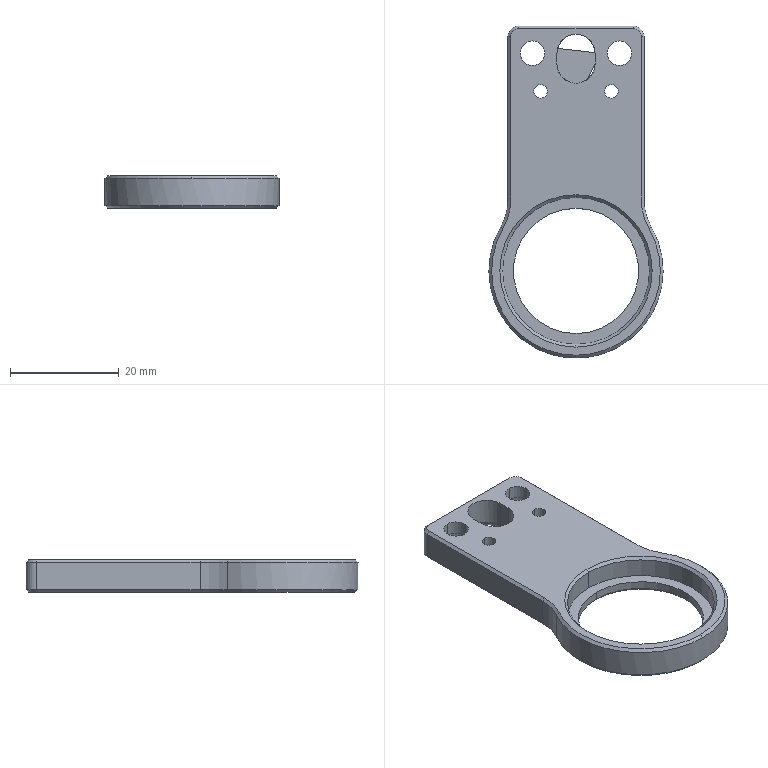Part | 1 solid | 75 faces | box 32 x 61 x 6 mm | volume 5137 mm3 | cylinder 32 | plane 18 | cone 15 | torus 6 | spline 4 | commonest cylinder face diameters 7 x7 4 x6 2.5 x4 4.5 x4 2 x3 20 x2